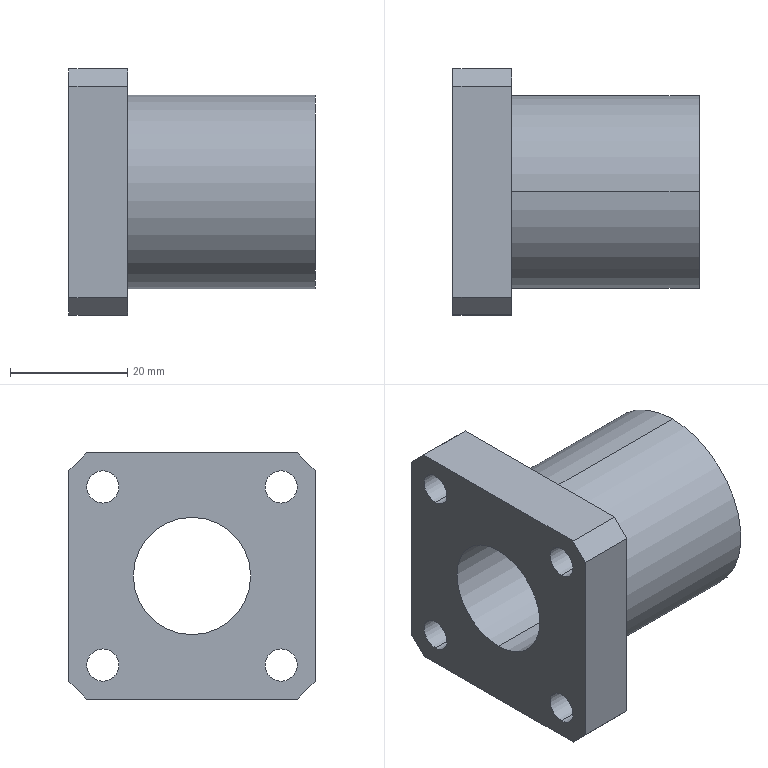Part | SolidWorks | features ICE 2, Chamfer 1, Extrusion 1, HoleWzd 1 | 1 solid | 23 faces | box 42 x 42 x 42 mm | volume 30685 mm3 | cylinder 12 | plane 11 | commonest cylinder face diameters 5.5 x8 20 x2 33 x2
STEP:
#1=CARTESIAN_POINT('',(42.,0.,-10.));
#2=VERTEX_POINT('',#1);
#3=CARTESIAN_POINT('',(42.,0.,10.));
#4=VERTEX_POINT('',#3);
#5=CARTESIAN_POINT('',(42.,0.,0.));
#6=DIRECTION('',(-1.,0.,0.));
#7=DIRECTION('',(0.,0.,1.));
#8=AXIS2_PLACEMENT_3D('',#5,#6,#7);
#9=CIRCLE('',#8,10.);
#10=EDGE_CURVE('',#2,#4,#9,.T.);
#11=ORIENTED_EDGE('',*,*,#10,.F.);
#12=CARTESIAN_POINT('',(0.,0.,-10.));
#13=VERTEX_POINT('',#12);
#14=CARTESIAN_POINT('',(42.,0.,-10.));
#15=DIRECTION('',(-1.,0.,0.));
#16=VECTOR('',#15,1000.);
#17=LINE('',#14,#16);
#18=EDGE_CURVE('',#2,#13,#17,.T.);
#19=ORIENTED_EDGE('',*,*,#18,.T.);
#20=CARTESIAN_POINT('',(0.,0.,10.));
#21=VERTEX_POINT('',#20);
#22=CARTESIAN_POINT('',(0.,0.,0.));
#23=DIRECTION('',(-1.,0.,0.));
#24=DIRECTION('',(0.,0.,1.));
#25=AXIS2_PLACEMENT_3D('',#22,#23,#24);
#26=CIRCLE('',#25,10.);
#27=EDGE_CURVE('',#13,#21,#26,.T.);
#28=ORIENTED_EDGE('',*,*,#27,.T.);
#29=CARTESIAN_POINT('',(42.,0.,10.));
#30=DIRECTION('',(-1.,0.,0.));
#31=VECTOR('',#30,1000.);
#32=LINE('',#29,#31);
#33=EDGE_CURVE('',#4,#21,#32,.T.);
#34=ORIENTED_EDGE('',*,*,#33,.F.);
#35=EDGE_LOOP('',(#11,#19,#28,#34));
#36=FACE_OUTER_BOUND('',#35,.T.);
#37=CARTESIAN_POINT('',(42.,0.,0.));
#38=DIRECTION('',(-1.,0.,0.));
#39=DIRECTION('',(0.,0.,1.));
#40=AXIS2_PLACEMENT_3D('',#37,#38,#39);
#41=CYLINDRICAL_SURFACE('',#40,10.);
#42=ADVANCED_FACE('',(#36),#41,.F.);
#43=CARTESIAN_POINT('',(10.,15.203,-12.453));
#44=VERTEX_POINT('',#43);
#45=CARTESIAN_POINT('',(10.,15.203,-17.953));
#46=VERTEX_POINT('',#45);
#47=CARTESIAN_POINT('',(10.,15.203,-15.203));
#48=DIRECTION('',(1.,0.,0.));
#49=DIRECTION('',(0.,0.,-1.));
#50=AXIS2_PLACEMENT_3D('',#47,#48,#49);
#51=CIRCLE('',#50,2.75);
#52=EDGE_CURVE('',#44,#46,#51,.T.);
#53=ORIENTED_EDGE('',*,*,#52,.T.);
#54=CARTESIAN_POINT('',(0.,15.203,-17.953));
#55=VERTEX_POINT('',#54);
#56=CARTESIAN_POINT('',(0.,15.203,-17.953));
#57=DIRECTION('',(-1.,0.,0.));
#58=VECTOR('',#57,1000.);
#59=LINE('',#56,#58);
#60=EDGE_CURVE('',#46,#55,#59,.T.);
#61=ORIENTED_EDGE('',*,*,#60,.T.);
#62=CARTESIAN_POINT('',(0.,15.203,-12.453));
#63=VERTEX_POINT('',#62);
#64=CARTESIAN_POINT('',(0.,15.203,-15.203));
#65=DIRECTION('',(-1.,0.,0.));
#66=DIRECTION('',(0.,0.,1.));
#67=AXIS2_PLACEMENT_3D('',#64,#65,#66);
#68=CIRCLE('',#67,2.75);
#69=EDGE_CURVE('',#55,#63,#68,.T.);
#70=ORIENTED_EDGE('',*,*,#69,.T.);
#71=CARTESIAN_POINT('',(0.,15.203,-12.453));
#72=DIRECTION('',(-1.,0.,0.));
#73=VECTOR('',#72,1000.);
#74=LINE('',#71,#73);
#75=EDGE_CURVE('',#44,#63,#74,.T.);
#76=ORIENTED_EDGE('',*,*,#75,.F.);
#77=EDGE_LOOP('',(#53,#61,#70,#76));
#78=FACE_OUTER_BOUND('',#77,.T.);
#79=CARTESIAN_POINT('',(0.,15.203,-15.203));
#80=DIRECTION('',(-1.,0.,0.));
#81=DIRECTION('',(0.,0.,1.));
#82=AXIS2_PLACEMENT_3D('',#79,#80,#81);
#83=CYLINDRICAL_SURFACE('',#82,2.75);
#84=ADVANCED_FACE('',(#78),#83,.F.);
#85=CARTESIAN_POINT('',(10.,15.203,17.953));
#86=VERTEX_POINT('',#85);
#87=CARTESIAN_POINT('',(10.,15.203,12.453));
#88=VERTEX_POINT('',#87);
#89=CARTESIAN_POINT('',(10.,15.203,15.203));
#90=DIRECTION('',(1.,0.,0.));
#91=DIRECTION('',(0.,0.,-1.));
#92=AXIS2_PLACEMENT_3D('',#89,#90,#91);
#93=CIRCLE('',#92,2.75);
#94=EDGE_CURVE('',#86,#88,#93,.T.);
#95=ORIENTED_EDGE('',*,*,#94,.T.);
#96=CARTESIAN_POINT('',(0.,15.203,12.453));
#97=VERTEX_POINT('',#96);
#98=CARTESIAN_POINT('',(0.,15.203,12.453));
#99=DIRECTION('',(-1.,0.,0.));
#100=VECTOR('',#99,1000.);
#101=LINE('',#98,#100);
#102=EDGE_CURVE('',#88,#97,#101,.T.);
#103=ORIENTED_EDGE('',*,*,#102,.T.);
#104=CARTESIAN_POINT('',(0.,15.203,17.953));
#105=VERTEX_POINT('',#104);
#106=CARTESIAN_POINT('',(0.,15.203,15.203));
#107=DIRECTION('',(-1.,0.,0.));
#108=DIRECTION('',(0.,0.,1.));
#109=AXIS2_PLACEMENT_3D('',#106,#107,#108);
#110=CIRCLE('',#109,2.75);
#111=EDGE_CURVE('',#97,#105,#110,.T.);
#112=ORIENTED_EDGE('',*,*,#111,.T.);
#113=CARTESIAN_POINT('',(0.,15.203,17.953));
#114=DIRECTION('',(-1.,0.,0.));
#115=VECTOR('',#114,1000.);
#116=LINE('',#113,#115);
#117=EDGE_CURVE('',#86,#105,#116,.T.);
#118=ORIENTED_EDGE('',*,*,#117,.F.);
#119=EDGE_LOOP('',(#95,#103,#112,#118));
#120=FACE_OUTER_BOUND('',#119,.T.);
#121=CARTESIAN_POINT('',(0.,15.203,15.203));
#122=DIRECTION('',(-1.,0.,0.));
#123=DIRECTION('',(0.,0.,1.));
#124=AXIS2_PLACEMENT_3D('',#121,#122,#123);
#125=CYLINDRICAL_SURFACE('',#124,2.75);
#126=ADVANCED_FACE('',(#120),#125,.F.);
#127=CARTESIAN_POINT('',(10.,-15.203,17.953));
#128=VERTEX_POINT('',#127);
#129=CARTESIAN_POINT('',(10.,-15.203,12.453));
#130=VERTEX_POINT('',#129);
#131=CARTESIAN_POINT('',(10.,-15.203,15.203));
#132=DIRECTION('',(1.,0.,0.));
#133=DIRECTION('',(0.,0.,-1.));
#134=AXIS2_PLACEMENT_3D('',#131,#132,#133);
#135=CIRCLE('',#134,2.75);
#136=EDGE_CURVE('',#128,#130,#135,.T.);
#137=ORIENTED_EDGE('',*,*,#136,.T.);
#138=CARTESIAN_POINT('',(0.,-15.203,12.453));
#139=VERTEX_POINT('',#138);
#140=CARTESIAN_POINT('',(0.,-15.203,12.453));
#141=DIRECTION('',(-1.,0.,0.));
#142=VECTOR('',#141,1000.);
#143=LINE('',#140,#142);
#144=EDGE_CURVE('',#130,#139,#143,.T.);
#145=ORIENTED_EDGE('',*,*,#144,.T.);
#146=CARTESIAN_POINT('',(0.,-15.203,17.953));
#147=VERTEX_POINT('',#146);
#148=CARTESIAN_POINT('',(0.,-15.203,15.203));
#149=DIRECTION('',(-1.,0.,0.));
#150=DIRECTION('',(0.,0.,1.));
#151=AXIS2_PLACEMENT_3D('',#148,#149,#150);
#152=CIRCLE('',#151,2.75);
#153=EDGE_CURVE('',#139,#147,#152,.T.);
#154=ORIENTED_EDGE('',*,*,#153,.T.);
#155=CARTESIAN_POINT('',(0.,-15.203,17.953));
#156=DIRECTION('',(-1.,0.,0.));
#157=VECTOR('',#156,1000.);
#158=LINE('',#155,#157);
#159=EDGE_CURVE('',#128,#147,#158,.T.);
#160=ORIENTED_EDGE('',*,*,#159,.F.);
#161=EDGE_LOOP('',(#137,#145,#154,#160));
#162=FACE_OUTER_BOUND('',#161,.T.);
#163=CARTESIAN_POINT('',(0.,-15.203,15.203));
#164=DIRECTION('',(-1.,0.,0.));
#165=DIRECTION('',(0.,0.,1.));
#166=AXIS2_PLACEMENT_3D('',#163,#164,#165);
#167=CYLINDRICAL_SURFACE('',#166,2.75);
#168=ADVANCED_FACE('',(#162),#167,.F.);
#169=CARTESIAN_POINT('',(10.,-15.203,-12.453));
#170=VERTEX_POINT('',#169);
#171=CARTESIAN_POINT('',(10.,-15.203,-17.953));
#172=VERTEX_POINT('',#171);
#173=CARTESIAN_POINT('',(10.,-15.203,-15.203));
#174=DIRECTION('',(1.,0.,0.));
#175=DIRECTION('',(0.,0.,-1.));
#176=AXIS2_PLACEMENT_3D('',#173,#174,#175);
#177=CIRCLE('',#176,2.75);
#178=EDGE_CURVE('',#170,#172,#177,.T.);
#179=ORIENTED_EDGE('',*,*,#178,.T.);
#180=CARTESIAN_POINT('',(0.,-15.203,-17.953));
#181=VERTEX_POINT('',#180);
#182=CARTESIAN_POINT('',(0.,-15.203,-17.953));
#183=DIRECTION('',(-1.,0.,0.));
#184=VECTOR('',#183,1000.);
#185=LINE('',#182,#184);
#186=EDGE_CURVE('',#172,#181,#185,.T.);
#187=ORIENTED_EDGE('',*,*,#186,.T.);
#188=CARTESIAN_POINT('',(0.,-15.203,-12.453));
#189=VERTEX_POINT('',#188);
#190=CARTESIAN_POINT('',(0.,-15.203,-15.203));
#191=DIRECTION('',(-1.,0.,0.));
#192=DIRECTION('',(0.,0.,1.));
#193=AXIS2_PLACEMENT_3D('',#190,#191,#192);
#194=CIRCLE('',#193,2.75);
#195=EDGE_CURVE('',#181,#189,#194,.T.);
#196=ORIENTED_EDGE('',*,*,#195,.T.);
#197=CARTESIAN_POINT('',(0.,-15.203,-12.453));
#198=DIRECTION('',(-1.,0.,0.));
#199=VECTOR('',#198,1000.);
#200=LINE('',#197,#199);
#201=EDGE_CURVE('',#170,#189,#200,.T.);
#202=ORIENTED_EDGE('',*,*,#201,.F.);
#203=EDGE_LOOP('',(#179,#187,#196,#202));
#204=FACE_OUTER_BOUND('',#203,.T.);
#205=CARTESIAN_POINT('',(0.,-15.203,-15.203));
#206=DIRECTION('',(-1.,0.,0.));
#207=DIRECTION('',(0.,0.,1.));
#208=AXIS2_PLACEMENT_3D('',#205,#206,#207);
#209=CYLINDRICAL_SURFACE('',#208,2.75);
#210=ADVANCED_FACE('',(#204),#209,.F.);
#211=CARTESIAN_POINT('',(42.,0.,-16.5));
#212=VERTEX_POINT('',#211);
#213=CARTESIAN_POINT('',(42.,0.,16.5));
#214=VERTEX_POINT('',#213);
#215=CARTESIAN_POINT('',(42.,0.,0.));
#216=DIRECTION('',(1.,0.,0.));
#217=DIRECTION('',(0.,0.,1.));
#218=AXIS2_PLACEMENT_3D('',#215,#216,#217);
#219=CIRCLE('',#218,16.5);
#220=EDGE_CURVE('',#212,#214,#219,.T.);
#221=ORIENTED_EDGE('',*,*,#220,.F.);
#222=CARTESIAN_POINT('',(10.,0.,-16.5));
#223=VERTEX_POINT('',#222);
#224=CARTESIAN_POINT('',(42.,0.,-16.5));
#225=DIRECTION('',(-1.,0.,0.));
#226=VECTOR('',#225,1000.);
#227=LINE('',#224,#226);
#228=EDGE_CURVE('',#212,#223,#227,.T.);
#229=ORIENTED_EDGE('',*,*,#228,.T.);
#230=CARTESIAN_POINT('',(10.,0.,16.5));
#231=VERTEX_POINT('',#230);
#232=CARTESIAN_POINT('',(10.,0.,0.));
#233=DIRECTION('',(1.,0.,0.));
#234=DIRECTION('',(0.,0.,1.));
#235=AXIS2_PLACEMENT_3D('',#232,#233,#234);
#236=CIRCLE('',#235,16.5);
#237=EDGE_CURVE('',#223,#231,#236,.T.);
#238=ORIENTED_EDGE('',*,*,#237,.T.);
#239=CARTESIAN_POINT('',(42.,0.,16.5));
#240=DIRECTION('',(-1.,0.,0.));
#241=VECTOR('',#240,1000.);
#242=LINE('',#239,#241);
#243=EDGE_CURVE('',#214,#231,#242,.T.);
#244=ORIENTED_EDGE('',*,*,#243,.F.);
#245=EDGE_LOOP('',(#221,#229,#238,#244));
#246=FACE_OUTER_BOUND('',#245,.T.);
#247=CARTESIAN_POINT('',(42.,0.,0.));
#248=DIRECTION('',(-1.,0.,0.));
#249=DIRECTION('',(0.,0.,1.));
#250=AXIS2_PLACEMENT_3D('',#247,#248,#249);
#251=CYLINDRICAL_SURFACE('',#250,16.5);
#252=ADVANCED_FACE('',(#246),#251,.T.);
#253=CARTESIAN_POINT('',(0.,0.,0.));
#254=DIRECTION('',(-1.,0.,0.));
#255=DIRECTION('',(0.,0.,1.));
#256=AXIS2_PLACEMENT_3D('',#253,#254,#255);
#257=CIRCLE('',#256,10.);
#258=EDGE_CURVE('',#21,#13,#257,.T.);
#259=ORIENTED_EDGE('',*,*,#258,.F.);
#260=ORIENTED_EDGE('',*,*,#27,.F.);
#261=EDGE_LOOP('',(#259,#260));
#262=FACE_BOUND('',#261,.T.);
#263=CARTESIAN_POINT('',(0.,15.203,-15.203));
#264=DIRECTION('',(-1.,0.,0.));
#265=DIRECTION('',(0.,0.,1.));
#266=AXIS2_PLACEMENT_3D('',#263,#264,#265);
#267=CIRCLE('',#266,2.75);
#268=EDGE_CURVE('',#63,#55,#267,.T.);
#269=ORIENTED_EDGE('',*,*,#268,.F.);
#270=ORIENTED_EDGE('',*,*,#69,.F.);
#271=EDGE_LOOP('',(#269,#270));
#272=FACE_BOUND('',#271,.T.);
#273=CARTESIAN_POINT('',(0.,-15.203,15.203));
#274=DIRECTION('',(-1.,0.,0.));
#275=DIRECTION('',(0.,0.,1.));
#276=AXIS2_PLACEMENT_3D('',#273,#274,#275);
#277=CIRCLE('',#276,2.75);
#278=EDGE_CURVE('',#147,#139,#277,.T.);
#279=ORIENTED_EDGE('',*,*,#278,.F.);
#280=ORIENTED_EDGE('',*,*,#153,.F.);
#281=EDGE_LOOP('',(#279,#280));
#282=FACE_BOUND('',#281,.T.);
#283=CARTESIAN_POINT('',(0.,-15.203,-15.203));
#284=DIRECTION('',(-1.,0.,0.));
#285=DIRECTION('',(0.,0.,1.));
#286=AXIS2_PLACEMENT_3D('',#283,#284,#285);
#287=CIRCLE('',#286,2.75);
#288=EDGE_CURVE('',#189,#181,#287,.T.);
#289=ORIENTED_EDGE('',*,*,#288,.F.);
#290=ORIENTED_EDGE('',*,*,#195,.F.);
#291=EDGE_LOOP('',(#289,#290));
#292=FACE_BOUND('',#291,.T.);
#293=CARTESIAN_POINT('',(0.,21.,-18.));
#294=VERTEX_POINT('',#293);
#295=CARTESIAN_POINT('',(0.,21.,18.));
#296=VERTEX_POINT('',#295);
#297=CARTESIAN_POINT('',(0.,21.,-21.));
#298=DIRECTION('',(0.,0.,1.));
#299=VECTOR('',#298,1000.);
#300=LINE('',#297,#299);
#301=EDGE_CURVE('',#294,#296,#300,.T.);
#302=ORIENTED_EDGE('',*,*,#301,.F.);
#303=CARTESIAN_POINT('',(0.,18.,-21.));
#304=VERTEX_POINT('',#303);
#305=CARTESIAN_POINT('',(0.,21.,-18.));
#306=DIRECTION('',(0.,-0.7071,-0.7071));
#307=VECTOR('',#306,1000.);
#308=LINE('',#305,#307);
#309=EDGE_CURVE('',#294,#304,#308,.T.);
#310=ORIENTED_EDGE('',*,*,#309,.T.);
#311=CARTESIAN_POINT('',(0.,-18.,-21.));
#312=VERTEX_POINT('',#311);
#313=CARTESIAN_POINT('',(0.,-21.,-21.));
#314=DIRECTION('',(0.,1.,0.));
#315=VECTOR('',#314,1000.);
#316=LINE('',#313,#315);
#317=EDGE_CURVE('',#312,#304,#316,.T.);
#318=ORIENTED_EDGE('',*,*,#317,.F.);
#319=CARTESIAN_POINT('',(0.,-21.,-18.));
#320=VERTEX_POINT('',#319);
#321=CARTESIAN_POINT('',(0.,-18.,-21.));
#322=DIRECTION('',(0.,-0.7071,0.7071));
#323=VECTOR('',#322,1000.);
#324=LINE('',#321,#323);
#325=EDGE_CURVE('',#312,#320,#324,.T.);
#326=ORIENTED_EDGE('',*,*,#325,.T.);
#327=CARTESIAN_POINT('',(0.,-21.,18.));
#328=VERTEX_POINT('',#327);
#329=CARTESIAN_POINT('',(0.,-21.,-21.));
#330=DIRECTION('',(0.,0.,-1.));
#331=VECTOR('',#330,1000.);
#332=LINE('',#329,#331);
#333=EDGE_CURVE('',#328,#320,#332,.T.);
#334=ORIENTED_EDGE('',*,*,#333,.F.);
#335=CARTESIAN_POINT('',(0.,-18.,21.));
#336=VERTEX_POINT('',#335);
#337=CARTESIAN_POINT('',(0.,-21.,18.));
#338=DIRECTION('',(0.,0.7071,0.7071));
#339=VECTOR('',#338,1000.);
#340=LINE('',#337,#339);
#341=EDGE_CURVE('',#328,#336,#340,.T.);
#342=ORIENTED_EDGE('',*,*,#341,.T.);
#343=CARTESIAN_POINT('',(0.,18.,21.));
#344=VERTEX_POINT('',#343);
#345=CARTESIAN_POINT('',(0.,21.,21.));
#346=DIRECTION('',(0.,-1.,0.));
#347=VECTOR('',#346,1000.);
#348=LINE('',#345,#347);
#349=EDGE_CURVE('',#344,#336,#348,.T.);
#350=ORIENTED_EDGE('',*,*,#349,.F.);
#351=CARTESIAN_POINT('',(0.,18.,21.));
#352=DIRECTION('',(0.,0.7071,-0.7071));
#353=VECTOR('',#352,1000.);
#354=LINE('',#351,#353);
#355=EDGE_CURVE('',#344,#296,#354,.T.);
#356=ORIENTED_EDGE('',*,*,#355,.T.);
#357=EDGE_LOOP('',(#302,#310,#318,#326,#334,#342,#350,#356));
#358=FACE_OUTER_BOUND('',#357,.T.);
#359=CARTESIAN_POINT('',(0.,15.203,15.203));
#360=DIRECTION('',(-1.,0.,0.));
#361=DIRECTION('',(0.,0.,1.));
#362=AXIS2_PLACEMENT_3D('',#359,#360,#361);
#363=CIRCLE('',#362,2.75);
#364=EDGE_CURVE('',#105,#97,#363,.T.);
#365=ORIENTED_EDGE('',*,*,#364,.F.);
#366=ORIENTED_EDGE('',*,*,#111,.F.);
#367=EDGE_LOOP('',(#365,#366));
#368=FACE_BOUND('',#367,.T.);
#369=CARTESIAN_POINT('',(0.,0.,0.));
#370=DIRECTION('',(1.,0.,0.));
#371=DIRECTION('',(0.,0.,-1.));
#372=AXIS2_PLACEMENT_3D('',#369,#370,#371);
#373=PLANE('',#372);
#374=ADVANCED_FACE('',(#262,#272,#282,#292,#358,#368),#373,.F.);
#375=CARTESIAN_POINT('',(10.,21.,-18.));
#376=VERTEX_POINT('',#375);
#377=CARTESIAN_POINT('',(10.,21.,18.));
#378=VERTEX_POINT('',#377);
#379=CARTESIAN_POINT('',(10.,21.,-21.));
#380=DIRECTION('',(0.,0.,1.));
#381=VECTOR('',#380,1000.);
#382=LINE('',#379,#381);
#383=EDGE_CURVE('',#376,#378,#382,.T.);
#384=ORIENTED_EDGE('',*,*,#383,.F.);
#385=CARTESIAN_POINT('',(10.,21.,-18.));
#386=DIRECTION('',(-1.,0.,0.));
#387=VECTOR('',#386,1000.);
#388=LINE('',#385,#387);
#389=EDGE_CURVE('',#376,#294,#388,.T.);
#390=ORIENTED_EDGE('',*,*,#389,.T.);
#391=ORIENTED_EDGE('',*,*,#301,.T.);
#392=CARTESIAN_POINT('',(10.,21.,18.));
#393=DIRECTION('',(1.,0.,0.));
#394=VECTOR('',#393,1000.);
#395=LINE('',#392,#394);
#396=EDGE_CURVE('',#296,#378,#395,.T.);
#397=ORIENTED_EDGE('',*,*,#396,.T.);
#398=EDGE_LOOP('',(#384,#390,#391,#397));
#399=FACE_OUTER_BOUND('',#398,.T.);
#400=CARTESIAN_POINT('',(10.,21.,-21.));
#401=DIRECTION('',(0.,-1.,0.));
#402=DIRECTION('',(0.,0.,-1.));
#403=AXIS2_PLACEMENT_3D('',#400,#401,#402);
#404=PLANE('',#403);
#405=ADVANCED_FACE('',(#399),#404,.F.);
#406=ORIENTED_EDGE('',*,*,#349,.T.);
#407=CARTESIAN_POINT('',(10.,-18.,21.));
#408=VERTEX_POINT('',#407);
#409=CARTESIAN_POINT('',(10.,-18.,21.));
#410=DIRECTION('',(1.,0.,0.));
#411=VECTOR('',#410,1000.);
#412=LINE('',#409,#411);
#413=EDGE_CURVE('',#336,#408,#412,.T.);
#414=ORIENTED_EDGE('',*,*,#413,.T.);
#415=CARTESIAN_POINT('',(10.,18.,21.));
#416=VERTEX_POINT('',#415);
#417=CARTESIAN_POINT('',(10.,21.,21.));
#418=DIRECTION('',(0.,-1.,0.));
#419=VECTOR('',#418,1000.);
#420=LINE('',#417,#419);
#421=EDGE_CURVE('',#416,#408,#420,.T.);
#422=ORIENTED_EDGE('',*,*,#421,.F.);
#423=CARTESIAN_POINT('',(10.,18.,21.));
#424=DIRECTION('',(-1.,0.,0.));
#425=VECTOR('',#424,1000.);
#426=LINE('',#423,#425);
#427=EDGE_CURVE('',#416,#344,#426,.T.);
#428=ORIENTED_EDGE('',*,*,#427,.T.);
#429=EDGE_LOOP('',(#406,#414,#422,#428));
#430=FACE_OUTER_BOUND('',#429,.T.);
#431=CARTESIAN_POINT('',(10.,21.,21.));
#432=DIRECTION('',(0.,0.,-1.));
#433=DIRECTION('',(0.,1.,0.));
#434=AXIS2_PLACEMENT_3D('',#431,#432,#433);
#435=PLANE('',#434);
#436=ADVANCED_FACE('',(#430),#435,.F.);
#437=ORIENTED_EDGE('',*,*,#333,.T.);
#438=CARTESIAN_POINT('',(10.,-21.,-18.));
#439=VERTEX_POINT('',#438);
#440=CARTESIAN_POINT('',(10.,-21.,-18.));
#441=DIRECTION('',(1.,0.,0.));
#442=VECTOR('',#441,1000.);
#443=LINE('',#440,#442);
#444=EDGE_CURVE('',#320,#439,#443,.T.);
#445=ORIENTED_EDGE('',*,*,#444,.T.);
#446=CARTESIAN_POINT('',(10.,-21.,18.));
#447=VERTEX_POINT('',#446);
#448=CARTESIAN_POINT('',(10.,-21.,-21.));
#449=DIRECTION('',(0.,0.,-1.));
#450=VECTOR('',#449,1000.);
#451=LINE('',#448,#450);
#452=EDGE_CURVE('',#447,#439,#451,.T.);
#453=ORIENTED_EDGE('',*,*,#452,.F.);
#454=CARTESIAN_POINT('',(10.,-21.,18.));
#455=DIRECTION('',(-1.,0.,0.));
#456=VECTOR('',#455,1000.);
#457=LINE('',#454,#456);
#458=EDGE_CURVE('',#447,#328,#457,.T.);
#459=ORIENTED_EDGE('',*,*,#458,.T.);
#460=EDGE_LOOP('',(#437,#445,#453,#459));
#461=FACE_OUTER_BOUND('',#460,.T.);
#462=CARTESIAN_POINT('',(10.,-21.,-21.));
#463=DIRECTION('',(0.,1.,0.));
#464=DIRECTION('',(0.,0.,1.));
#465=AXIS2_PLACEMENT_3D('',#462,#463,#464);
#466=PLANE('',#465);
#467=ADVANCED_FACE('',(#461),#466,.F.);
#468=ORIENTED_EDGE('',*,*,#317,.T.);
#469=CARTESIAN_POINT('',(10.,18.,-21.));
#470=VERTEX_POINT('',#469);
#471=CARTESIAN_POINT('',(10.,18.,-21.));
#472=DIRECTION('',(1.,0.,0.));
#473=VECTOR('',#472,1000.);
#474=LINE('',#471,#473);
#475=EDGE_CURVE('',#304,#470,#474,.T.);
#476=ORIENTED_EDGE('',*,*,#475,.T.);
#477=CARTESIAN_POINT('',(10.,-18.,-21.));
#478=VERTEX_POINT('',#477);
#479=CARTESIAN_POINT('',(10.,-21.,-21.));
#480=DIRECTION('',(0.,1.,0.));
#481=VECTOR('',#480,1000.);
#482=LINE('',#479,#481);
#483=EDGE_CURVE('',#478,#470,#482,.T.);
#484=ORIENTED_EDGE('',*,*,#483,.F.);
#485=CARTESIAN_POINT('',(10.,-18.,-21.));
#486=DIRECTION('',(-1.,0.,0.));
#487=VECTOR('',#486,1000.);
#488=LINE('',#485,#487);
#489=EDGE_CURVE('',#478,#312,#488,.T.);
#490=ORIENTED_EDGE('',*,*,#489,.T.);
#491=EDGE_LOOP('',(#468,#476,#484,#490));
#492=FACE_OUTER_BOUND('',#491,.T.);
#493=CARTESIAN_POINT('',(10.,-21.,-21.));
#494=DIRECTION('',(0.,0.,1.));
#495=DIRECTION('',(0.,-1.,0.));
#496=AXIS2_PLACEMENT_3D('',#493,#494,#495);
#497=PLANE('',#496);
#498=ADVANCED_FACE('',(#492),#497,.F.);
#499=ORIENTED_EDGE('',*,*,#52,.F.);
#500=CARTESIAN_POINT('',(10.,15.203,-15.203));
#501=DIRECTION('',(1.,0.,0.));
#502=DIRECTION('',(0.,0.,-1.));
#503=AXIS2_PLACEMENT_3D('',#500,#501,#502);
#504=CIRCLE('',#503,2.75);
#505=EDGE_CURVE('',#46,#44,#504,.T.);
#506=ORIENTED_EDGE('',*,*,#505,.F.);
#507=EDGE_LOOP('',(#499,#506));
#508=FACE_BOUND('',#507,.T.);
#509=ORIENTED_EDGE('',*,*,#94,.F.);
#510=CARTESIAN_POINT('',(10.,15.203,15.203));
#511=DIRECTION('',(1.,0.,0.));
#512=DIRECTION('',(0.,0.,-1.));
#513=AXIS2_PLACEMENT_3D('',#510,#511,#512);
#514=CIRCLE('',#513,2.75);
#515=EDGE_CURVE('',#88,#86,#514,.T.);
#516=ORIENTED_EDGE('',*,*,#515,.F.);
#517=EDGE_LOOP('',(#509,#516));
#518=FACE_BOUND('',#517,.T.);
#519=ORIENTED_EDGE('',*,*,#136,.F.);
#520=CARTESIAN_POINT('',(10.,-15.203,15.203));
#521=DIRECTION('',(1.,0.,0.));
#522=DIRECTION('',(0.,0.,-1.));
#523=AXIS2_PLACEMENT_3D('',#520,#521,#522);
#524=CIRCLE('',#523,2.75);
#525=EDGE_CURVE('',#130,#128,#524,.T.);
#526=ORIENTED_EDGE('',*,*,#525,.F.);
#527=EDGE_LOOP('',(#519,#526));
#528=FACE_BOUND('',#527,.T.);
#529=ORIENTED_EDGE('',*,*,#178,.F.);
#530=CARTESIAN_POINT('',(10.,-15.203,-15.203));
#531=DIRECTION('',(1.,0.,0.));
#532=DIRECTION('',(0.,0.,-1.));
#533=AXIS2_PLACEMENT_3D('',#530,#531,#532);
#534=CIRCLE('',#533,2.75);
#535=EDGE_CURVE('',#172,#170,#534,.T.);
#536=ORIENTED_EDGE('',*,*,#535,.F.);
#537=EDGE_LOOP('',(#529,#536));
#538=FACE_BOUND('',#537,.T.);
#539=CARTESIAN_POINT('',(10.,0.,0.));
#540=DIRECTION('',(1.,0.,0.));
#541=DIRECTION('',(0.,0.,1.));
#542=AXIS2_PLACEMENT_3D('',#539,#540,#541);
#543=CIRCLE('',#542,16.5);
#544=EDGE_CURVE('',#231,#223,#543,.T.);
#545=ORIENTED_EDGE('',*,*,#544,.F.);
#546=ORIENTED_EDGE('',*,*,#237,.F.);
#547=EDGE_LOOP('',(#545,#546));
#548=FACE_BOUND('',#547,.T.);
#549=ORIENTED_EDGE('',*,*,#483,.T.);
#550=CARTESIAN_POINT('',(10.,19.5,-19.5));
#551=DIRECTION('',(0.,0.7071,0.7071));
#552=VECTOR('',#551,1000.);
#553=LINE('',#550,#552);
#554=EDGE_CURVE('',#470,#376,#553,.T.);
#555=ORIENTED_EDGE('',*,*,#554,.T.);
#556=ORIENTED_EDGE('',*,*,#383,.T.);
#557=CARTESIAN_POINT('',(10.,19.5,19.5));
#558=DIRECTION('',(0.,-0.7071,0.7071));
#559=VECTOR('',#558,1000.);
#560=LINE('',#557,#559);
#561=EDGE_CURVE('',#378,#416,#560,.T.);
#562=ORIENTED_EDGE('',*,*,#561,.T.);
#563=ORIENTED_EDGE('',*,*,#421,.T.);
#564=CARTESIAN_POINT('',(10.,-19.5,19.5));
#565=DIRECTION('',(0.,-0.7071,-0.7071));
#566=VECTOR('',#565,1000.);
#567=LINE('',#564,#566);
#568=EDGE_CURVE('',#408,#447,#567,.T.);
#569=ORIENTED_EDGE('',*,*,#568,.T.);
#570=ORIENTED_EDGE('',*,*,#452,.T.);
#571=CARTESIAN_POINT('',(10.,-19.5,-19.5));
#572=DIRECTION('',(0.,0.7071,-0.7071));
#573=VECTOR('',#572,1000.);
#574=LINE('',#571,#573);
#575=EDGE_CURVE('',#439,#478,#574,.T.);
#576=ORIENTED_EDGE('',*,*,#575,.T.);
#577=EDGE_LOOP('',(#549,#555,#556,#562,#563,#569,#570,#576));
#578=FACE_OUTER_BOUND('',#577,.T.);
#579=CARTESIAN_POINT('',(10.,0.,0.));
#580=DIRECTION('',(1.,0.,0.));
#581=DIRECTION('',(0.,0.,-1.));
#582=AXIS2_PLACEMENT_3D('',#579,#580,#581);
#583=PLANE('',#582);
#584=ADVANCED_FACE('',(#508,#518,#528,#538,#548,#578),#583,.T.);
#585=ORIENTED_EDGE('',*,*,#228,.F.);
#586=CARTESIAN_POINT('',(42.,0.,0.));
#587=DIRECTION('',(1.,0.,0.));
#588=DIRECTION('',(0.,0.,1.));
#589=AXIS2_PLACEMENT_3D('',#586,#587,#588);
#590=CIRCLE('',#589,16.5);
#591=EDGE_CURVE('',#214,#212,#590,.T.);
#592=ORIENTED_EDGE('',*,*,#591,.F.);
#593=ORIENTED_EDGE('',*,*,#243,.T.);
#594=ORIENTED_EDGE('',*,*,#544,.T.);
#595=EDGE_LOOP('',(#585,#592,#593,#594));
#596=FACE_OUTER_BOUND('',#595,.T.);
#597=CARTESIAN_POINT('',(42.,0.,0.));
#598=DIRECTION('',(-1.,0.,0.));
#599=DIRECTION('',(0.,0.,1.));
#600=AXIS2_PLACEMENT_3D('',#597,#598,#599);
#601=CYLINDRICAL_SURFACE('',#600,16.5);
#602=ADVANCED_FACE('',(#596),#601,.T.);
#603=CARTESIAN_POINT('',(42.,0.,0.));
#604=DIRECTION('',(-1.,0.,0.));
#605=DIRECTION('',(0.,0.,1.));
#606=AXIS2_PLACEMENT_3D('',#603,#604,#605);
#607=CIRCLE('',#606,10.);
#608=EDGE_CURVE('',#4,#2,#607,.T.);
#609=ORIENTED_EDGE('',*,*,#608,.T.);
#610=ORIENTED_EDGE('',*,*,#10,.T.);
#611=EDGE_LOOP('',(#609,#610));
#612=FACE_BOUND('',#611,.T.);
#613=ORIENTED_EDGE('',*,*,#591,.T.);
#614=ORIENTED_EDGE('',*,*,#220,.T.);
#615=EDGE_LOOP('',(#613,#614));
#616=FACE_OUTER_BOUND('',#615,.T.);
#617=CARTESIAN_POINT('',(42.,0.,0.));
#618=DIRECTION('',(-1.,0.,0.));
#619=DIRECTION('',(0.,0.,1.));
#620=AXIS2_PLACEMENT_3D('',#617,#618,#619);
#621=PLANE('',#620);
#622=ADVANCED_FACE('',(#612,#616),#621,.F.);
#623=ORIENTED_EDGE('',*,*,#186,.F.);
#624=ORIENTED_EDGE('',*,*,#535,.T.);
#625=ORIENTED_EDGE('',*,*,#201,.T.);
#626=ORIENTED_EDGE('',*,*,#288,.T.);
#627=EDGE_LOOP('',(#623,#624,#625,#626));
#628=FACE_OUTER_BOUND('',#627,.T.);
#629=CARTESIAN_POINT('',(0.,-15.203,-15.203));
#630=DIRECTION('',(-1.,0.,0.));
#631=DIRECTION('',(0.,0.,1.));
#632=AXIS2_PLACEMENT_3D('',#629,#630,#631);
#633=CYLINDRICAL_SURFACE('',#632,2.75);
#634=ADVANCED_FACE('',(#628),#633,.F.);
#635=ORIENTED_EDGE('',*,*,#144,.F.);
#636=ORIENTED_EDGE('',*,*,#525,.T.);
#637=ORIENTED_EDGE('',*,*,#159,.T.);
#638=ORIENTED_EDGE('',*,*,#278,.T.);
#639=EDGE_LOOP('',(#635,#636,#637,#638));
#640=FACE_OUTER_BOUND('',#639,.T.);
#641=CARTESIAN_POINT('',(0.,-15.203,15.203));
#642=DIRECTION('',(-1.,0.,0.));
#643=DIRECTION('',(0.,0.,1.));
#644=AXIS2_PLACEMENT_3D('',#641,#642,#643);
#645=CYLINDRICAL_SURFACE('',#644,2.75);
#646=ADVANCED_FACE('',(#640),#645,.F.);
#647=ORIENTED_EDGE('',*,*,#102,.F.);
#648=ORIENTED_EDGE('',*,*,#515,.T.);
#649=ORIENTED_EDGE('',*,*,#117,.T.);
#650=ORIENTED_EDGE('',*,*,#364,.T.);
#651=EDGE_LOOP('',(#647,#648,#649,#650));
#652=FACE_OUTER_BOUND('',#651,.T.);
#653=CARTESIAN_POINT('',(0.,15.203,15.203));
#654=DIRECTION('',(-1.,0.,0.));
#655=DIRECTION('',(0.,0.,1.));
#656=AXIS2_PLACEMENT_3D('',#653,#654,#655);
#657=CYLINDRICAL_SURFACE('',#656,2.75);
#658=ADVANCED_FACE('',(#652),#657,.F.);
#659=ORIENTED_EDGE('',*,*,#60,.F.);
#660=ORIENTED_EDGE('',*,*,#505,.T.);
#661=ORIENTED_EDGE('',*,*,#75,.T.);
#662=ORIENTED_EDGE('',*,*,#268,.T.);
#663=EDGE_LOOP('',(#659,#660,#661,#662));
#664=FACE_OUTER_BOUND('',#663,.T.);
#665=CARTESIAN_POINT('',(0.,15.203,-15.203));
#666=DIRECTION('',(-1.,0.,0.));
#667=DIRECTION('',(0.,0.,1.));
#668=AXIS2_PLACEMENT_3D('',#665,#666,#667);
#669=CYLINDRICAL_SURFACE('',#668,2.75);
#670=ADVANCED_FACE('',(#664),#669,.F.);
#671=ORIENTED_EDGE('',*,*,#18,.F.);
#672=ORIENTED_EDGE('',*,*,#608,.F.);
#673=ORIENTED_EDGE('',*,*,#33,.T.);
#674=ORIENTED_EDGE('',*,*,#258,.T.);
#675=EDGE_LOOP('',(#671,#672,#673,#674));
#676=FACE_OUTER_BOUND('',#675,.T.);
#677=CARTESIAN_POINT('',(42.,0.,0.));
#678=DIRECTION('',(-1.,0.,0.));
#679=DIRECTION('',(0.,0.,1.));
#680=AXIS2_PLACEMENT_3D('',#677,#678,#679);
#681=CYLINDRICAL_SURFACE('',#680,10.);
#682=ADVANCED_FACE('',(#676),#681,.F.);
#683=ORIENTED_EDGE('',*,*,#554,.F.);
#684=ORIENTED_EDGE('',*,*,#475,.F.);
#685=ORIENTED_EDGE('',*,*,#309,.F.);
#686=ORIENTED_EDGE('',*,*,#389,.F.);
#687=EDGE_LOOP('',(#683,#684,#685,#686));
#688=FACE_OUTER_BOUND('',#687,.T.);
#689=CARTESIAN_POINT('',(10.,21.,-18.));
#690=DIRECTION('',(0.,-0.7071,0.7071));
#691=DIRECTION('',(-1.,0.,0.));
#692=AXIS2_PLACEMENT_3D('',#689,#690,#691);
#693=PLANE('',#692);
#694=ADVANCED_FACE('',(#688),#693,.F.);
#695=ORIENTED_EDGE('',*,*,#575,.F.);
#696=ORIENTED_EDGE('',*,*,#444,.F.);
#697=ORIENTED_EDGE('',*,*,#325,.F.);
#698=ORIENTED_EDGE('',*,*,#489,.F.);
#699=EDGE_LOOP('',(#695,#696,#697,#698));
#700=FACE_OUTER_BOUND('',#699,.T.);
#701=CARTESIAN_POINT('',(10.,-18.,-21.));
#702=DIRECTION('',(0.,0.7071,0.7071));
#703=DIRECTION('',(-1.,0.,0.));
#704=AXIS2_PLACEMENT_3D('',#701,#702,#703);
#705=PLANE('',#704);
#706=ADVANCED_FACE('',(#700),#705,.F.);
#707=ORIENTED_EDGE('',*,*,#568,.F.);
#708=ORIENTED_EDGE('',*,*,#413,.F.);
#709=ORIENTED_EDGE('',*,*,#341,.F.);
#710=ORIENTED_EDGE('',*,*,#458,.F.);
#711=EDGE_LOOP('',(#707,#708,#709,#710));
#712=FACE_OUTER_BOUND('',#711,.T.);
#713=CARTESIAN_POINT('',(10.,-21.,18.));
#714=DIRECTION('',(0.,0.7071,-0.7071));
#715=DIRECTION('',(-1.,0.,0.));
#716=AXIS2_PLACEMENT_3D('',#713,#714,#715);
#717=PLANE('',#716);
#718=ADVANCED_FACE('',(#712),#717,.F.);
#719=ORIENTED_EDGE('',*,*,#561,.F.);
#720=ORIENTED_EDGE('',*,*,#396,.F.);
#721=ORIENTED_EDGE('',*,*,#355,.F.);
#722=ORIENTED_EDGE('',*,*,#427,.F.);
#723=EDGE_LOOP('',(#719,#720,#721,#722));
#724=FACE_OUTER_BOUND('',#723,.T.);
#725=CARTESIAN_POINT('',(10.,18.,21.));
#726=DIRECTION('',(0.,-0.7071,-0.7071));
#727=DIRECTION('',(-1.,0.,0.));
#728=AXIS2_PLACEMENT_3D('',#725,#726,#727);
#729=PLANE('',#728);
#730=ADVANCED_FACE('',(#724),#729,.F.);
#731=CLOSED_SHELL('',(#42,#84,#126,#168,#210,#252,#374,#405,#436,#467,#498,#584,#602,#622,#634,#646,#658,#670,#682,#694,#706,#718,#730));
#732=MANIFOLD_SOLID_BREP('',#731);
#733=CARTESIAN_POINT('',(0.,0.,0.));
#734=DIRECTION('',(0.,0.,1.));
#735=DIRECTION('',(1.,0.,0.));
#736=AXIS2_PLACEMENT_3D('',#733,#734,#735);
#737=(LENGTH_UNIT()NAMED_UNIT(*)SI_UNIT(.MILLI.,.METRE.));
#738=UNCERTAINTY_MEASURE_WITH_UNIT(LENGTH_MEASURE(0.00001),#737,'','');
#739=(NAMED_UNIT(*)PLANE_ANGLE_UNIT()SI_UNIT($,.RADIAN.));
#740=(NAMED_UNIT(*)SI_UNIT($,.STERADIAN.)SOLID_ANGLE_UNIT());
#741=(GEOMETRIC_REPRESENTATION_CONTEXT(3)GLOBAL_UNCERTAINTY_ASSIGNED_CONTEXT((#738))GLOBAL_UNIT_ASSIGNED_CONTEXT((#737,#739,#740))REPRESENTATION_CONTEXT('',''));
#742=ADVANCED_BREP_SHAPE_REPRESENTATION('',(#732,#736),#741);